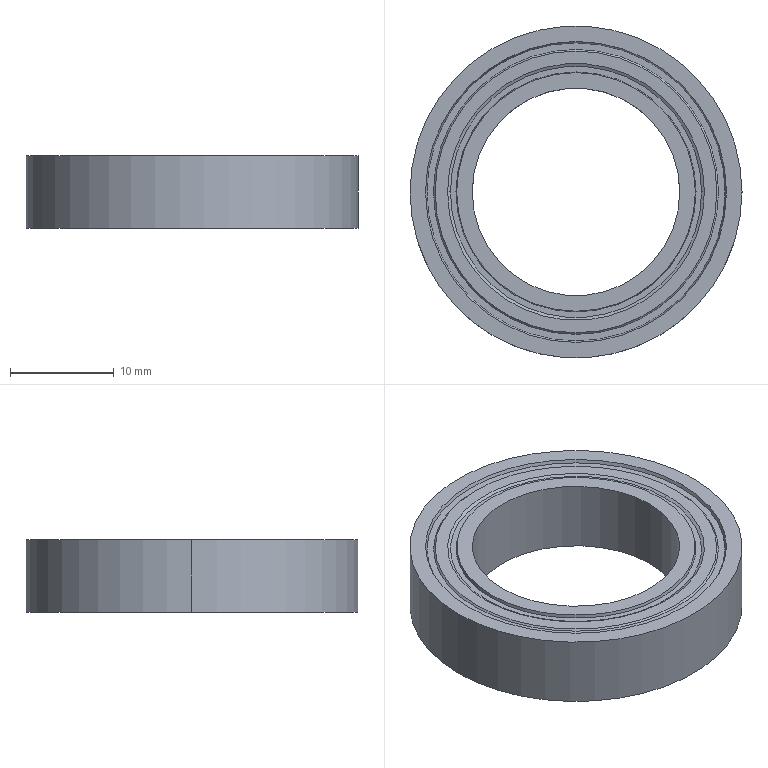Part | SolidWorks | features Extrusion 1, MirrorPattern 1, RevCut 1 | 1 solid | 30 faces | box 32 x 32 x 7 mm | volume 3321 mm3 | cone 16 | plane 10 | cylinder 4 | commonest cylinder face diameters 20 x2 32 x2
STEP:
#1=CARTESIAN_POINT('',(11.5,0.,0.));
#2=VERTEX_POINT('',#1);
#3=CARTESIAN_POINT('',(-11.5,0.,0.));
#4=VERTEX_POINT('',#3);
#5=CARTESIAN_POINT('',(0.,0.,0.));
#6=DIRECTION('',(0.,0.,-1.));
#7=DIRECTION('',(-1.,0.,0.));
#8=AXIS2_PLACEMENT_3D('',#5,#6,#7);
#9=CIRCLE('',#8,11.5);
#10=EDGE_CURVE('',#2,#4,#9,.T.);
#11=ORIENTED_EDGE('',*,*,#10,.F.);
#12=CARTESIAN_POINT('',(11.567,0.,0.3054));
#13=VERTEX_POINT('',#12);
#14=CARTESIAN_POINT('',(11.567,0.,0.3054));
#15=DIRECTION('',(0.215,0.,0.9766));
#16=VECTOR('',#15,1000.);
#17=LINE('',#14,#16);
#18=EDGE_CURVE('',#2,#13,#17,.T.);
#19=ORIENTED_EDGE('',*,*,#18,.T.);
#20=CARTESIAN_POINT('',(-11.567,0.,0.3054));
#21=VERTEX_POINT('',#20);
#22=CARTESIAN_POINT('',(0.,0.,0.3054));
#23=DIRECTION('',(0.,0.,-1.));
#24=DIRECTION('',(-1.,0.,0.));
#25=AXIS2_PLACEMENT_3D('',#22,#23,#24);
#26=CIRCLE('',#25,11.567);
#27=EDGE_CURVE('',#13,#21,#26,.T.);
#28=ORIENTED_EDGE('',*,*,#27,.T.);
#29=CARTESIAN_POINT('',(-11.567,0.,0.3054));
#30=DIRECTION('',(-0.215,0.,0.9766));
#31=VECTOR('',#30,1000.);
#32=LINE('',#29,#31);
#33=EDGE_CURVE('',#4,#21,#32,.T.);
#34=ORIENTED_EDGE('',*,*,#33,.F.);
#35=EDGE_LOOP('',(#11,#19,#28,#34));
#36=FACE_OUTER_BOUND('',#35,.T.);
#37=CARTESIAN_POINT('',(0.,0.,0.3054));
#38=DIRECTION('',(0.,0.,1.));
#39=DIRECTION('',(-1.,0.,0.));
#40=AXIS2_PLACEMENT_3D('',#37,#38,#39);
#41=CONICAL_SURFACE('',#40,11.567,0.2167);
#42=ADVANCED_FACE('',(#36),#41,.T.);
#43=CARTESIAN_POINT('',(-12.105,0.,0.3054));
#44=VERTEX_POINT('',#43);
#45=CARTESIAN_POINT('',(12.105,0.,0.3054));
#46=VERTEX_POINT('',#45);
#47=CARTESIAN_POINT('',(0.,0.,0.3054));
#48=DIRECTION('',(0.,0.,-1.));
#49=DIRECTION('',(-1.,0.,0.));
#50=AXIS2_PLACEMENT_3D('',#47,#48,#49);
#51=CIRCLE('',#50,12.105);
#52=EDGE_CURVE('',#44,#46,#51,.T.);
#53=ORIENTED_EDGE('',*,*,#52,.F.);
#54=CARTESIAN_POINT('',(-12.375,0.,0.1527));
#55=VERTEX_POINT('',#54);
#56=CARTESIAN_POINT('',(-12.375,0.,0.1527));
#57=DIRECTION('',(-0.8699,0.,-0.4932));
#58=VECTOR('',#57,1000.);
#59=LINE('',#56,#58);
#60=EDGE_CURVE('',#44,#55,#59,.T.);
#61=ORIENTED_EDGE('',*,*,#60,.T.);
#62=CARTESIAN_POINT('',(12.375,0.,0.1527));
#63=VERTEX_POINT('',#62);
#64=CARTESIAN_POINT('',(0.,0.,0.1527));
#65=DIRECTION('',(0.,0.,-1.));
#66=DIRECTION('',(-1.,0.,0.));
#67=AXIS2_PLACEMENT_3D('',#64,#65,#66);
#68=CIRCLE('',#67,12.375);
#69=EDGE_CURVE('',#55,#63,#68,.T.);
#70=ORIENTED_EDGE('',*,*,#69,.T.);
#71=CARTESIAN_POINT('',(12.375,0.,0.1527));
#72=DIRECTION('',(0.8699,0.,-0.4932));
#73=VECTOR('',#72,1000.);
#74=LINE('',#71,#73);
#75=EDGE_CURVE('',#46,#63,#74,.T.);
#76=ORIENTED_EDGE('',*,*,#75,.F.);
#77=EDGE_LOOP('',(#53,#61,#70,#76));
#78=FACE_OUTER_BOUND('',#77,.T.);
#79=CARTESIAN_POINT('',(0.,0.,0.1527));
#80=DIRECTION('',(0.,0.,-1.));
#81=DIRECTION('',(1.,0.,0.));
#82=AXIS2_PLACEMENT_3D('',#79,#80,#81);
#83=CONICAL_SURFACE('',#82,12.375,1.055);
#84=ADVANCED_FACE('',(#78),#83,.F.);
#85=CARTESIAN_POINT('',(13.575,0.,0.1527));
#86=VERTEX_POINT('',#85);
#87=CARTESIAN_POINT('',(-13.575,0.,0.1527));
#88=VERTEX_POINT('',#87);
#89=CARTESIAN_POINT('',(0.,0.,0.1527));
#90=DIRECTION('',(0.,0.,-1.));
#91=DIRECTION('',(-1.,0.,0.));
#92=AXIS2_PLACEMENT_3D('',#89,#90,#91);
#93=CIRCLE('',#92,13.575);
#94=EDGE_CURVE('',#86,#88,#93,.T.);
#95=ORIENTED_EDGE('',*,*,#94,.F.);
#96=CARTESIAN_POINT('',(13.727,0.,0.3054));
#97=VERTEX_POINT('',#96);
#98=CARTESIAN_POINT('',(13.727,0.,0.3054));
#99=DIRECTION('',(0.7071,0.,0.7071));
#100=VECTOR('',#99,1000.);
#101=LINE('',#98,#100);
#102=EDGE_CURVE('',#86,#97,#101,.T.);
#103=ORIENTED_EDGE('',*,*,#102,.T.);
#104=CARTESIAN_POINT('',(-13.727,0.,0.3054));
#105=VERTEX_POINT('',#104);
#106=CARTESIAN_POINT('',(0.,0.,0.3054));
#107=DIRECTION('',(0.,0.,-1.));
#108=DIRECTION('',(-1.,0.,0.));
#109=AXIS2_PLACEMENT_3D('',#106,#107,#108);
#110=CIRCLE('',#109,13.727);
#111=EDGE_CURVE('',#97,#105,#110,.T.);
#112=ORIENTED_EDGE('',*,*,#111,.T.);
#113=CARTESIAN_POINT('',(-13.727,0.,0.3054));
#114=DIRECTION('',(-0.7071,0.,0.7071));
#115=VECTOR('',#114,1000.);
#116=LINE('',#113,#115);
#117=EDGE_CURVE('',#88,#105,#116,.T.);
#118=ORIENTED_EDGE('',*,*,#117,.F.);
#119=EDGE_LOOP('',(#95,#103,#112,#118));
#120=FACE_OUTER_BOUND('',#119,.T.);
#121=CARTESIAN_POINT('',(0.,0.,0.3054));
#122=DIRECTION('',(0.,0.,1.));
#123=DIRECTION('',(-1.,0.,0.));
#124=AXIS2_PLACEMENT_3D('',#121,#122,#123);
#125=CONICAL_SURFACE('',#124,13.727,0.7854);
#126=ADVANCED_FACE('',(#120),#125,.T.);
#127=CARTESIAN_POINT('',(-14.366,0.,0.3054));
#128=VERTEX_POINT('',#127);
#129=CARTESIAN_POINT('',(14.366,0.,0.3054));
#130=VERTEX_POINT('',#129);
#131=CARTESIAN_POINT('',(0.,0.,0.3054));
#132=DIRECTION('',(0.,0.,-1.));
#133=DIRECTION('',(-1.,0.,0.));
#134=AXIS2_PLACEMENT_3D('',#131,#132,#133);
#135=CIRCLE('',#134,14.366);
#136=EDGE_CURVE('',#128,#130,#135,.T.);
#137=ORIENTED_EDGE('',*,*,#136,.F.);
#138=CARTESIAN_POINT('',(-14.5,0.,0.));
#139=VERTEX_POINT('',#138);
#140=CARTESIAN_POINT('',(-14.5,0.,0.));
#141=DIRECTION('',(-0.4019,0.,-0.9157));
#142=VECTOR('',#141,1000.);
#143=LINE('',#140,#142);
#144=EDGE_CURVE('',#128,#139,#143,.T.);
#145=ORIENTED_EDGE('',*,*,#144,.T.);
#146=CARTESIAN_POINT('',(14.5,0.,0.));
#147=VERTEX_POINT('',#146);
#148=CARTESIAN_POINT('',(0.,0.,0.));
#149=DIRECTION('',(0.,0.,-1.));
#150=DIRECTION('',(-1.,0.,0.));
#151=AXIS2_PLACEMENT_3D('',#148,#149,#150);
#152=CIRCLE('',#151,14.5);
#153=EDGE_CURVE('',#139,#147,#152,.T.);
#154=ORIENTED_EDGE('',*,*,#153,.T.);
#155=CARTESIAN_POINT('',(14.5,0.,0.));
#156=DIRECTION('',(0.4019,0.,-0.9157));
#157=VECTOR('',#156,1000.);
#158=LINE('',#155,#157);
#159=EDGE_CURVE('',#130,#147,#158,.T.);
#160=ORIENTED_EDGE('',*,*,#159,.F.);
#161=EDGE_LOOP('',(#137,#145,#154,#160));
#162=FACE_OUTER_BOUND('',#161,.T.);
#163=CARTESIAN_POINT('',(0.,0.,0.));
#164=DIRECTION('',(0.,0.,-1.));
#165=DIRECTION('',(1.,0.,0.));
#166=AXIS2_PLACEMENT_3D('',#163,#164,#165);
#167=CONICAL_SURFACE('',#166,14.5,0.4136);
#168=ADVANCED_FACE('',(#162),#167,.F.);
#169=CARTESIAN_POINT('',(-11.5,0.,7.));
#170=VERTEX_POINT('',#169);
#171=CARTESIAN_POINT('',(11.5,0.,7.));
#172=VERTEX_POINT('',#171);
#173=CARTESIAN_POINT('',(0.,0.,7.));
#174=DIRECTION('',(0.,0.,-1.));
#175=DIRECTION('',(-1.,0.,0.));
#176=AXIS2_PLACEMENT_3D('',#173,#174,#175);
#177=CIRCLE('',#176,11.5);
#178=EDGE_CURVE('',#170,#172,#177,.T.);
#179=ORIENTED_EDGE('',*,*,#178,.T.);
#180=CARTESIAN_POINT('',(11.567,0.,6.695));
#181=VERTEX_POINT('',#180);
#182=CARTESIAN_POINT('',(11.567,0.,6.695));
#183=DIRECTION('',(0.215,0.,-0.9766));
#184=VECTOR('',#183,1000.);
#185=LINE('',#182,#184);
#186=EDGE_CURVE('',#172,#181,#185,.T.);
#187=ORIENTED_EDGE('',*,*,#186,.T.);
#188=CARTESIAN_POINT('',(-11.567,0.,6.695));
#189=VERTEX_POINT('',#188);
#190=CARTESIAN_POINT('',(0.,0.,6.695));
#191=DIRECTION('',(0.,0.,-1.));
#192=DIRECTION('',(-1.,0.,0.));
#193=AXIS2_PLACEMENT_3D('',#190,#191,#192);
#194=CIRCLE('',#193,11.567);
#195=EDGE_CURVE('',#189,#181,#194,.T.);
#196=ORIENTED_EDGE('',*,*,#195,.F.);
#197=CARTESIAN_POINT('',(-11.567,0.,6.695));
#198=DIRECTION('',(-0.215,0.,-0.9766));
#199=VECTOR('',#198,1000.);
#200=LINE('',#197,#199);
#201=EDGE_CURVE('',#170,#189,#200,.T.);
#202=ORIENTED_EDGE('',*,*,#201,.F.);
#203=EDGE_LOOP('',(#179,#187,#196,#202));
#204=FACE_OUTER_BOUND('',#203,.T.);
#205=CARTESIAN_POINT('',(0.,0.,6.695));
#206=DIRECTION('',(0.,0.,-1.));
#207=DIRECTION('',(-1.,0.,0.));
#208=AXIS2_PLACEMENT_3D('',#205,#206,#207);
#209=CONICAL_SURFACE('',#208,11.567,0.2167);
#210=ADVANCED_FACE('',(#204),#209,.T.);
#211=CARTESIAN_POINT('',(12.105,0.,6.695));
#212=VERTEX_POINT('',#211);
#213=CARTESIAN_POINT('',(-12.105,0.,6.695));
#214=VERTEX_POINT('',#213);
#215=CARTESIAN_POINT('',(0.,0.,6.695));
#216=DIRECTION('',(0.,0.,-1.));
#217=DIRECTION('',(-1.,0.,0.));
#218=AXIS2_PLACEMENT_3D('',#215,#216,#217);
#219=CIRCLE('',#218,12.105);
#220=EDGE_CURVE('',#212,#214,#219,.T.);
#221=ORIENTED_EDGE('',*,*,#220,.T.);
#222=CARTESIAN_POINT('',(-12.375,0.,6.847));
#223=VERTEX_POINT('',#222);
#224=CARTESIAN_POINT('',(-12.375,0.,6.847));
#225=DIRECTION('',(-0.8699,0.,0.4932));
#226=VECTOR('',#225,1000.);
#227=LINE('',#224,#226);
#228=EDGE_CURVE('',#214,#223,#227,.T.);
#229=ORIENTED_EDGE('',*,*,#228,.T.);
#230=CARTESIAN_POINT('',(12.375,0.,6.847));
#231=VERTEX_POINT('',#230);
#232=CARTESIAN_POINT('',(0.,0.,6.847));
#233=DIRECTION('',(0.,0.,-1.));
#234=DIRECTION('',(-1.,0.,0.));
#235=AXIS2_PLACEMENT_3D('',#232,#233,#234);
#236=CIRCLE('',#235,12.375);
#237=EDGE_CURVE('',#231,#223,#236,.T.);
#238=ORIENTED_EDGE('',*,*,#237,.F.);
#239=CARTESIAN_POINT('',(12.375,0.,6.847));
#240=DIRECTION('',(0.8699,0.,0.4932));
#241=VECTOR('',#240,1000.);
#242=LINE('',#239,#241);
#243=EDGE_CURVE('',#212,#231,#242,.T.);
#244=ORIENTED_EDGE('',*,*,#243,.F.);
#245=EDGE_LOOP('',(#221,#229,#238,#244));
#246=FACE_OUTER_BOUND('',#245,.T.);
#247=CARTESIAN_POINT('',(0.,0.,6.847));
#248=DIRECTION('',(0.,0.,1.));
#249=DIRECTION('',(1.,0.,0.));
#250=AXIS2_PLACEMENT_3D('',#247,#248,#249);
#251=CONICAL_SURFACE('',#250,12.375,1.055);
#252=ADVANCED_FACE('',(#246),#251,.F.);
#253=CARTESIAN_POINT('',(-13.575,0.,6.847));
#254=VERTEX_POINT('',#253);
#255=CARTESIAN_POINT('',(13.575,0.,6.847));
#256=VERTEX_POINT('',#255);
#257=CARTESIAN_POINT('',(0.,0.,6.847));
#258=DIRECTION('',(0.,0.,-1.));
#259=DIRECTION('',(-1.,0.,0.));
#260=AXIS2_PLACEMENT_3D('',#257,#258,#259);
#261=CIRCLE('',#260,13.575);
#262=EDGE_CURVE('',#254,#256,#261,.T.);
#263=ORIENTED_EDGE('',*,*,#262,.T.);
#264=CARTESIAN_POINT('',(13.727,0.,6.695));
#265=VERTEX_POINT('',#264);
#266=CARTESIAN_POINT('',(13.727,0.,6.695));
#267=DIRECTION('',(0.7071,0.,-0.7071));
#268=VECTOR('',#267,1000.);
#269=LINE('',#266,#268);
#270=EDGE_CURVE('',#256,#265,#269,.T.);
#271=ORIENTED_EDGE('',*,*,#270,.T.);
#272=CARTESIAN_POINT('',(-13.727,0.,6.695));
#273=VERTEX_POINT('',#272);
#274=CARTESIAN_POINT('',(0.,0.,6.695));
#275=DIRECTION('',(0.,0.,-1.));
#276=DIRECTION('',(-1.,0.,0.));
#277=AXIS2_PLACEMENT_3D('',#274,#275,#276);
#278=CIRCLE('',#277,13.727);
#279=EDGE_CURVE('',#273,#265,#278,.T.);
#280=ORIENTED_EDGE('',*,*,#279,.F.);
#281=CARTESIAN_POINT('',(-13.727,0.,6.695));
#282=DIRECTION('',(-0.7071,0.,-0.7071));
#283=VECTOR('',#282,1000.);
#284=LINE('',#281,#283);
#285=EDGE_CURVE('',#254,#273,#284,.T.);
#286=ORIENTED_EDGE('',*,*,#285,.F.);
#287=EDGE_LOOP('',(#263,#271,#280,#286));
#288=FACE_OUTER_BOUND('',#287,.T.);
#289=CARTESIAN_POINT('',(0.,0.,6.695));
#290=DIRECTION('',(0.,0.,-1.));
#291=DIRECTION('',(-1.,0.,0.));
#292=AXIS2_PLACEMENT_3D('',#289,#290,#291);
#293=CONICAL_SURFACE('',#292,13.727,0.7854);
#294=ADVANCED_FACE('',(#288),#293,.T.);
#295=CARTESIAN_POINT('',(14.366,0.,6.695));
#296=VERTEX_POINT('',#295);
#297=CARTESIAN_POINT('',(-14.366,0.,6.695));
#298=VERTEX_POINT('',#297);
#299=CARTESIAN_POINT('',(0.,0.,6.695));
#300=DIRECTION('',(0.,0.,-1.));
#301=DIRECTION('',(-1.,0.,0.));
#302=AXIS2_PLACEMENT_3D('',#299,#300,#301);
#303=CIRCLE('',#302,14.366);
#304=EDGE_CURVE('',#296,#298,#303,.T.);
#305=ORIENTED_EDGE('',*,*,#304,.T.);
#306=CARTESIAN_POINT('',(-14.5,0.,7.));
#307=VERTEX_POINT('',#306);
#308=CARTESIAN_POINT('',(-14.5,0.,7.));
#309=DIRECTION('',(-0.4019,0.,0.9157));
#310=VECTOR('',#309,1000.);
#311=LINE('',#308,#310);
#312=EDGE_CURVE('',#298,#307,#311,.T.);
#313=ORIENTED_EDGE('',*,*,#312,.T.);
#314=CARTESIAN_POINT('',(14.5,0.,7.));
#315=VERTEX_POINT('',#314);
#316=CARTESIAN_POINT('',(0.,0.,7.));
#317=DIRECTION('',(0.,0.,-1.));
#318=DIRECTION('',(-1.,0.,0.));
#319=AXIS2_PLACEMENT_3D('',#316,#317,#318);
#320=CIRCLE('',#319,14.5);
#321=EDGE_CURVE('',#315,#307,#320,.T.);
#322=ORIENTED_EDGE('',*,*,#321,.F.);
#323=CARTESIAN_POINT('',(14.5,0.,7.));
#324=DIRECTION('',(0.4019,0.,0.9157));
#325=VECTOR('',#324,1000.);
#326=LINE('',#323,#325);
#327=EDGE_CURVE('',#296,#315,#326,.T.);
#328=ORIENTED_EDGE('',*,*,#327,.F.);
#329=EDGE_LOOP('',(#305,#313,#322,#328));
#330=FACE_OUTER_BOUND('',#329,.T.);
#331=CARTESIAN_POINT('',(0.,0.,7.));
#332=DIRECTION('',(0.,0.,1.));
#333=DIRECTION('',(1.,0.,0.));
#334=AXIS2_PLACEMENT_3D('',#331,#332,#333);
#335=CONICAL_SURFACE('',#334,14.5,0.4136);
#336=ADVANCED_FACE('',(#330),#335,.F.);
#337=CARTESIAN_POINT('',(-10.,0.,7.));
#338=VERTEX_POINT('',#337);
#339=CARTESIAN_POINT('',(10.,0.,7.));
#340=VERTEX_POINT('',#339);
#341=CARTESIAN_POINT('',(0.,0.,7.));
#342=DIRECTION('',(0.,0.,1.));
#343=DIRECTION('',(1.,0.,0.));
#344=AXIS2_PLACEMENT_3D('',#341,#342,#343);
#345=CIRCLE('',#344,10.);
#346=EDGE_CURVE('',#338,#340,#345,.T.);
#347=ORIENTED_EDGE('',*,*,#346,.T.);
#348=CARTESIAN_POINT('',(10.,0.,0.));
#349=VERTEX_POINT('',#348);
#350=CARTESIAN_POINT('',(10.,0.,7.));
#351=DIRECTION('',(0.,0.,-1.));
#352=VECTOR('',#351,1000.);
#353=LINE('',#350,#352);
#354=EDGE_CURVE('',#340,#349,#353,.T.);
#355=ORIENTED_EDGE('',*,*,#354,.T.);
#356=CARTESIAN_POINT('',(-10.,0.,0.));
#357=VERTEX_POINT('',#356);
#358=CARTESIAN_POINT('',(0.,0.,0.));
#359=DIRECTION('',(0.,0.,1.));
#360=DIRECTION('',(1.,0.,0.));
#361=AXIS2_PLACEMENT_3D('',#358,#359,#360);
#362=CIRCLE('',#361,10.);
#363=EDGE_CURVE('',#357,#349,#362,.T.);
#364=ORIENTED_EDGE('',*,*,#363,.F.);
#365=CARTESIAN_POINT('',(-10.,0.,7.));
#366=DIRECTION('',(0.,0.,-1.));
#367=VECTOR('',#366,1000.);
#368=LINE('',#365,#367);
#369=EDGE_CURVE('',#338,#357,#368,.T.);
#370=ORIENTED_EDGE('',*,*,#369,.F.);
#371=EDGE_LOOP('',(#347,#355,#364,#370));
#372=FACE_OUTER_BOUND('',#371,.T.);
#373=CARTESIAN_POINT('',(0.,0.,7.));
#374=DIRECTION('',(0.,0.,-1.));
#375=DIRECTION('',(-1.,0.,0.));
#376=AXIS2_PLACEMENT_3D('',#373,#374,#375);
#377=CYLINDRICAL_SURFACE('',#376,10.);
#378=ADVANCED_FACE('',(#372),#377,.F.);
#379=CARTESIAN_POINT('',(16.,0.,7.));
#380=VERTEX_POINT('',#379);
#381=CARTESIAN_POINT('',(-16.,0.,7.));
#382=VERTEX_POINT('',#381);
#383=CARTESIAN_POINT('',(0.,0.,7.));
#384=DIRECTION('',(0.,0.,1.));
#385=DIRECTION('',(1.,0.,0.));
#386=AXIS2_PLACEMENT_3D('',#383,#384,#385);
#387=CIRCLE('',#386,16.);
#388=EDGE_CURVE('',#380,#382,#387,.T.);
#389=ORIENTED_EDGE('',*,*,#388,.F.);
#390=CARTESIAN_POINT('',(16.,0.,0.));
#391=VERTEX_POINT('',#390);
#392=CARTESIAN_POINT('',(16.,0.,7.));
#393=DIRECTION('',(0.,0.,-1.));
#394=VECTOR('',#393,1000.);
#395=LINE('',#392,#394);
#396=EDGE_CURVE('',#380,#391,#395,.T.);
#397=ORIENTED_EDGE('',*,*,#396,.T.);
#398=CARTESIAN_POINT('',(-16.,0.,0.));
#399=VERTEX_POINT('',#398);
#400=CARTESIAN_POINT('',(0.,0.,0.));
#401=DIRECTION('',(0.,0.,1.));
#402=DIRECTION('',(1.,0.,0.));
#403=AXIS2_PLACEMENT_3D('',#400,#401,#402);
#404=CIRCLE('',#403,16.);
#405=EDGE_CURVE('',#391,#399,#404,.T.);
#406=ORIENTED_EDGE('',*,*,#405,.T.);
#407=CARTESIAN_POINT('',(-16.,0.,7.));
#408=DIRECTION('',(0.,0.,-1.));
#409=VECTOR('',#408,1000.);
#410=LINE('',#407,#409);
#411=EDGE_CURVE('',#382,#399,#410,.T.);
#412=ORIENTED_EDGE('',*,*,#411,.F.);
#413=EDGE_LOOP('',(#389,#397,#406,#412));
#414=FACE_OUTER_BOUND('',#413,.T.);
#415=CARTESIAN_POINT('',(0.,0.,7.));
#416=DIRECTION('',(0.,0.,-1.));
#417=DIRECTION('',(-1.,0.,0.));
#418=AXIS2_PLACEMENT_3D('',#415,#416,#417);
#419=CYLINDRICAL_SURFACE('',#418,16.);
#420=ADVANCED_FACE('',(#414),#419,.T.);
#421=CARTESIAN_POINT('',(0.,0.,0.));
#422=DIRECTION('',(0.,0.,1.));
#423=DIRECTION('',(1.,0.,0.));
#424=AXIS2_PLACEMENT_3D('',#421,#422,#423);
#425=CIRCLE('',#424,16.);
#426=EDGE_CURVE('',#399,#391,#425,.T.);
#427=ORIENTED_EDGE('',*,*,#426,.F.);
#428=ORIENTED_EDGE('',*,*,#405,.F.);
#429=EDGE_LOOP('',(#427,#428));
#430=FACE_OUTER_BOUND('',#429,.T.);
#431=CARTESIAN_POINT('',(0.,0.,0.));
#432=DIRECTION('',(0.,0.,-1.));
#433=DIRECTION('',(-1.,0.,0.));
#434=AXIS2_PLACEMENT_3D('',#431,#432,#433);
#435=CIRCLE('',#434,14.5);
#436=EDGE_CURVE('',#147,#139,#435,.T.);
#437=ORIENTED_EDGE('',*,*,#436,.F.);
#438=ORIENTED_EDGE('',*,*,#153,.F.);
#439=EDGE_LOOP('',(#437,#438));
#440=FACE_BOUND('',#439,.T.);
#441=CARTESIAN_POINT('',(0.,0.,0.));
#442=DIRECTION('',(0.,0.,1.));
#443=DIRECTION('',(1.,0.,0.));
#444=AXIS2_PLACEMENT_3D('',#441,#442,#443);
#445=PLANE('',#444);
#446=ADVANCED_FACE('',(#430,#440),#445,.F.);
#447=ORIENTED_EDGE('',*,*,#363,.T.);
#448=CARTESIAN_POINT('',(0.,0.,0.));
#449=DIRECTION('',(0.,0.,1.));
#450=DIRECTION('',(1.,0.,0.));
#451=AXIS2_PLACEMENT_3D('',#448,#449,#450);
#452=CIRCLE('',#451,10.);
#453=EDGE_CURVE('',#349,#357,#452,.T.);
#454=ORIENTED_EDGE('',*,*,#453,.T.);
#455=EDGE_LOOP('',(#447,#454));
#456=FACE_BOUND('',#455,.T.);
#457=CARTESIAN_POINT('',(0.,0.,0.));
#458=DIRECTION('',(0.,0.,-1.));
#459=DIRECTION('',(-1.,0.,0.));
#460=AXIS2_PLACEMENT_3D('',#457,#458,#459);
#461=CIRCLE('',#460,11.5);
#462=EDGE_CURVE('',#4,#2,#461,.T.);
#463=ORIENTED_EDGE('',*,*,#462,.T.);
#464=ORIENTED_EDGE('',*,*,#10,.T.);
#465=EDGE_LOOP('',(#463,#464));
#466=FACE_OUTER_BOUND('',#465,.T.);
#467=CARTESIAN_POINT('',(0.,0.,0.));
#468=DIRECTION('',(0.,0.,1.));
#469=DIRECTION('',(1.,0.,0.));
#470=AXIS2_PLACEMENT_3D('',#467,#468,#469);
#471=PLANE('',#470);
#472=ADVANCED_FACE('',(#456,#466),#471,.F.);
#473=CARTESIAN_POINT('',(0.,0.,7.));
#474=DIRECTION('',(0.,0.,1.));
#475=DIRECTION('',(1.,0.,0.));
#476=AXIS2_PLACEMENT_3D('',#473,#474,#475);
#477=CIRCLE('',#476,16.);
#478=EDGE_CURVE('',#382,#380,#477,.T.);
#479=ORIENTED_EDGE('',*,*,#478,.T.);
#480=ORIENTED_EDGE('',*,*,#388,.T.);
#481=EDGE_LOOP('',(#479,#480));
#482=FACE_OUTER_BOUND('',#481,.T.);
#483=ORIENTED_EDGE('',*,*,#321,.T.);
#484=CARTESIAN_POINT('',(0.,0.,7.));
#485=DIRECTION('',(0.,0.,-1.));
#486=DIRECTION('',(-1.,0.,0.));
#487=AXIS2_PLACEMENT_3D('',#484,#485,#486);
#488=CIRCLE('',#487,14.5);
#489=EDGE_CURVE('',#307,#315,#488,.T.);
#490=ORIENTED_EDGE('',*,*,#489,.T.);
#491=EDGE_LOOP('',(#483,#490));
#492=FACE_BOUND('',#491,.T.);
#493=CARTESIAN_POINT('',(0.,0.,7.));
#494=DIRECTION('',(0.,0.,1.));
#495=DIRECTION('',(1.,0.,0.));
#496=AXIS2_PLACEMENT_3D('',#493,#494,#495);
#497=PLANE('',#496);
#498=ADVANCED_FACE('',(#482,#492),#497,.T.);
#499=ORIENTED_EDGE('',*,*,#346,.F.);
#500=CARTESIAN_POINT('',(0.,0.,7.));
#501=DIRECTION('',(0.,0.,1.));
#502=DIRECTION('',(1.,0.,0.));
#503=AXIS2_PLACEMENT_3D('',#500,#501,#502);
#504=CIRCLE('',#503,10.);
#505=EDGE_CURVE('',#340,#338,#504,.T.);
#506=ORIENTED_EDGE('',*,*,#505,.F.);
#507=EDGE_LOOP('',(#499,#506));
#508=FACE_BOUND('',#507,.T.);
#509=ORIENTED_EDGE('',*,*,#178,.F.);
#510=CARTESIAN_POINT('',(0.,0.,7.));
#511=DIRECTION('',(0.,0.,-1.));
#512=DIRECTION('',(-1.,0.,0.));
#513=AXIS2_PLACEMENT_3D('',#510,#511,#512);
#514=CIRCLE('',#513,11.5);
#515=EDGE_CURVE('',#172,#170,#514,.T.);
#516=ORIENTED_EDGE('',*,*,#515,.F.);
#517=EDGE_LOOP('',(#509,#516));
#518=FACE_OUTER_BOUND('',#517,.T.);
#519=CARTESIAN_POINT('',(0.,0.,7.));
#520=DIRECTION('',(0.,0.,1.));
#521=DIRECTION('',(1.,0.,0.));
#522=AXIS2_PLACEMENT_3D('',#519,#520,#521);
#523=PLANE('',#522);
#524=ADVANCED_FACE('',(#508,#518),#523,.T.);
#525=ORIENTED_EDGE('',*,*,#396,.F.);
#526=ORIENTED_EDGE('',*,*,#478,.F.);
#527=ORIENTED_EDGE('',*,*,#411,.T.);
#528=ORIENTED_EDGE('',*,*,#426,.T.);
#529=EDGE_LOOP('',(#525,#526,#527,#528));
#530=FACE_OUTER_BOUND('',#529,.T.);
#531=CARTESIAN_POINT('',(0.,0.,7.));
#532=DIRECTION('',(0.,0.,-1.));
#533=DIRECTION('',(-1.,0.,0.));
#534=AXIS2_PLACEMENT_3D('',#531,#532,#533);
#535=CYLINDRICAL_SURFACE('',#534,16.);
#536=ADVANCED_FACE('',(#530),#535,.T.);
#537=ORIENTED_EDGE('',*,*,#354,.F.);
#538=ORIENTED_EDGE('',*,*,#505,.T.);
#539=ORIENTED_EDGE('',*,*,#369,.T.);
#540=ORIENTED_EDGE('',*,*,#453,.F.);
#541=EDGE_LOOP('',(#537,#538,#539,#540));
#542=FACE_OUTER_BOUND('',#541,.T.);
#543=CARTESIAN_POINT('',(0.,0.,7.));
#544=DIRECTION('',(0.,0.,-1.));
#545=DIRECTION('',(-1.,0.,0.));
#546=AXIS2_PLACEMENT_3D('',#543,#544,#545);
#547=CYLINDRICAL_SURFACE('',#546,10.);
#548=ADVANCED_FACE('',(#542),#547,.F.);
#549=ORIENTED_EDGE('',*,*,#312,.F.);
#550=CARTESIAN_POINT('',(0.,0.,6.695));
#551=DIRECTION('',(0.,0.,-1.));
#552=DIRECTION('',(-1.,0.,0.));
#553=AXIS2_PLACEMENT_3D('',#550,#551,#552);
#554=CIRCLE('',#553,14.366);
#555=EDGE_CURVE('',#298,#296,#554,.T.);
#556=ORIENTED_EDGE('',*,*,#555,.T.);
#557=ORIENTED_EDGE('',*,*,#327,.T.);
#558=ORIENTED_EDGE('',*,*,#489,.F.);
#559=EDGE_LOOP('',(#549,#556,#557,#558));
#560=FACE_OUTER_BOUND('',#559,.T.);
#561=CARTESIAN_POINT('',(0.,0.,7.));
#562=DIRECTION('',(0.,0.,1.));
#563=DIRECTION('',(1.,0.,0.));
#564=AXIS2_PLACEMENT_3D('',#561,#562,#563);
#565=CONICAL_SURFACE('',#564,14.5,0.4136);
#566=ADVANCED_FACE('',(#560),#565,.F.);
#567=ORIENTED_EDGE('',*,*,#279,.T.);
#568=CARTESIAN_POINT('',(0.,0.,6.695));
#569=DIRECTION('',(0.,0.,-1.));
#570=DIRECTION('',(-1.,0.,0.));
#571=AXIS2_PLACEMENT_3D('',#568,#569,#570);
#572=CIRCLE('',#571,13.727);
#573=EDGE_CURVE('',#265,#273,#572,.T.);
#574=ORIENTED_EDGE('',*,*,#573,.T.);
#575=EDGE_LOOP('',(#567,#574));
#576=FACE_BOUND('',#575,.T.);
#577=ORIENTED_EDGE('',*,*,#304,.F.);
#578=ORIENTED_EDGE('',*,*,#555,.F.);
#579=EDGE_LOOP('',(#577,#578));
#580=FACE_OUTER_BOUND('',#579,.T.);
#581=CARTESIAN_POINT('',(13.727,0.,6.695));
#582=DIRECTION('',(0.,0.,1.));
#583=DIRECTION('',(1.,0.,0.));
#584=AXIS2_PLACEMENT_3D('',#581,#582,#583);
#585=PLANE('',#584);
#586=ADVANCED_FACE('',(#576,#580),#585,.T.);
#587=ORIENTED_EDGE('',*,*,#270,.F.);
#588=CARTESIAN_POINT('',(0.,0.,6.847));
#589=DIRECTION('',(0.,0.,-1.));
#590=DIRECTION('',(-1.,0.,0.));
#591=AXIS2_PLACEMENT_3D('',#588,#589,#590);
#592=CIRCLE('',#591,13.575);
#593=EDGE_CURVE('',#256,#254,#592,.T.);
#594=ORIENTED_EDGE('',*,*,#593,.T.);
#595=ORIENTED_EDGE('',*,*,#285,.T.);
#596=ORIENTED_EDGE('',*,*,#573,.F.);
#597=EDGE_LOOP('',(#587,#594,#595,#596));
#598=FACE_OUTER_BOUND('',#597,.T.);
#599=CARTESIAN_POINT('',(0.,0.,6.695));
#600=DIRECTION('',(0.,0.,-1.));
#601=DIRECTION('',(-1.,0.,0.));
#602=AXIS2_PLACEMENT_3D('',#599,#600,#601);
#603=CONICAL_SURFACE('',#602,13.727,0.7854);
#604=ADVANCED_FACE('',(#598),#603,.T.);
#605=ORIENTED_EDGE('',*,*,#237,.T.);
#606=CARTESIAN_POINT('',(0.,0.,6.847));
#607=DIRECTION('',(0.,0.,-1.));
#608=DIRECTION('',(-1.,0.,0.));
#609=AXIS2_PLACEMENT_3D('',#606,#607,#608);
#610=CIRCLE('',#609,12.375);
#611=EDGE_CURVE('',#223,#231,#610,.T.);
#612=ORIENTED_EDGE('',*,*,#611,.T.);
#613=EDGE_LOOP('',(#605,#612));
#614=FACE_BOUND('',#613,.T.);
#615=ORIENTED_EDGE('',*,*,#262,.F.);
#616=ORIENTED_EDGE('',*,*,#593,.F.);
#617=EDGE_LOOP('',(#615,#616));
#618=FACE_OUTER_BOUND('',#617,.T.);
#619=CARTESIAN_POINT('',(12.375,0.,6.847));
#620=DIRECTION('',(0.,0.,1.));
#621=DIRECTION('',(1.,0.,0.));
#622=AXIS2_PLACEMENT_3D('',#619,#620,#621);
#623=PLANE('',#622);
#624=ADVANCED_FACE('',(#614,#618),#623,.T.);
#625=ORIENTED_EDGE('',*,*,#228,.F.);
#626=CARTESIAN_POINT('',(0.,0.,6.695));
#627=DIRECTION('',(0.,0.,-1.));
#628=DIRECTION('',(-1.,0.,0.));
#629=AXIS2_PLACEMENT_3D('',#626,#627,#628);
#630=CIRCLE('',#629,12.105);
#631=EDGE_CURVE('',#214,#212,#630,.T.);
#632=ORIENTED_EDGE('',*,*,#631,.T.);
#633=ORIENTED_EDGE('',*,*,#243,.T.);
#634=ORIENTED_EDGE('',*,*,#611,.F.);
#635=EDGE_LOOP('',(#625,#632,#633,#634));
#636=FACE_OUTER_BOUND('',#635,.T.);
#637=CARTESIAN_POINT('',(0.,0.,6.847));
#638=DIRECTION('',(0.,0.,1.));
#639=DIRECTION('',(1.,0.,0.));
#640=AXIS2_PLACEMENT_3D('',#637,#638,#639);
#641=CONICAL_SURFACE('',#640,12.375,1.055);
#642=ADVANCED_FACE('',(#636),#641,.F.);
#643=ORIENTED_EDGE('',*,*,#195,.T.);
#644=CARTESIAN_POINT('',(0.,0.,6.695));
#645=DIRECTION('',(0.,0.,-1.));
#646=DIRECTION('',(-1.,0.,0.));
#647=AXIS2_PLACEMENT_3D('',#644,#645,#646);
#648=CIRCLE('',#647,11.567);
#649=EDGE_CURVE('',#181,#189,#648,.T.);
#650=ORIENTED_EDGE('',*,*,#649,.T.);
#651=EDGE_LOOP('',(#643,#650));
#652=FACE_BOUND('',#651,.T.);
#653=ORIENTED_EDGE('',*,*,#220,.F.);
#654=ORIENTED_EDGE('',*,*,#631,.F.);
#655=EDGE_LOOP('',(#653,#654));
#656=FACE_OUTER_BOUND('',#655,.T.);
#657=CARTESIAN_POINT('',(11.567,0.,6.695));
#658=DIRECTION('',(0.,0.,1.));
#659=DIRECTION('',(1.,0.,0.));
#660=AXIS2_PLACEMENT_3D('',#657,#658,#659);
#661=PLANE('',#660);
#662=ADVANCED_FACE('',(#652,#656),#661,.T.);
#663=ORIENTED_EDGE('',*,*,#186,.F.);
#664=ORIENTED_EDGE('',*,*,#515,.T.);
#665=ORIENTED_EDGE('',*,*,#201,.T.);
#666=ORIENTED_EDGE('',*,*,#649,.F.);
#667=EDGE_LOOP('',(#663,#664,#665,#666));
#668=FACE_OUTER_BOUND('',#667,.T.);
#669=CARTESIAN_POINT('',(0.,0.,6.695));
#670=DIRECTION('',(0.,0.,-1.));
#671=DIRECTION('',(-1.,0.,0.));
#672=AXIS2_PLACEMENT_3D('',#669,#670,#671);
#673=CONICAL_SURFACE('',#672,11.567,0.2167);
#674=ADVANCED_FACE('',(#668),#673,.T.);
#675=ORIENTED_EDGE('',*,*,#144,.F.);
#676=CARTESIAN_POINT('',(0.,0.,0.3054));
#677=DIRECTION('',(0.,0.,-1.));
#678=DIRECTION('',(-1.,0.,0.));
#679=AXIS2_PLACEMENT_3D('',#676,#677,#678);
#680=CIRCLE('',#679,14.366);
#681=EDGE_CURVE('',#130,#128,#680,.T.);
#682=ORIENTED_EDGE('',*,*,#681,.F.);
#683=ORIENTED_EDGE('',*,*,#159,.T.);
#684=ORIENTED_EDGE('',*,*,#436,.T.);
#685=EDGE_LOOP('',(#675,#682,#683,#684));
#686=FACE_OUTER_BOUND('',#685,.T.);
#687=CARTESIAN_POINT('',(0.,0.,0.));
#688=DIRECTION('',(0.,0.,-1.));
#689=DIRECTION('',(1.,0.,0.));
#690=AXIS2_PLACEMENT_3D('',#687,#688,#689);
#691=CONICAL_SURFACE('',#690,14.5,0.4136);
#692=ADVANCED_FACE('',(#686),#691,.F.);
#693=CARTESIAN_POINT('',(0.,0.,0.3054));
#694=DIRECTION('',(0.,0.,-1.));
#695=DIRECTION('',(-1.,0.,0.));
#696=AXIS2_PLACEMENT_3D('',#693,#694,#695);
#697=CIRCLE('',#696,13.727);
#698=EDGE_CURVE('',#105,#97,#697,.T.);
#699=ORIENTED_EDGE('',*,*,#698,.F.);
#700=ORIENTED_EDGE('',*,*,#111,.F.);
#701=EDGE_LOOP('',(#699,#700));
#702=FACE_BOUND('',#701,.T.);
#703=ORIENTED_EDGE('',*,*,#681,.T.);
#704=ORIENTED_EDGE('',*,*,#136,.T.);
#705=EDGE_LOOP('',(#703,#704));
#706=FACE_OUTER_BOUND('',#705,.T.);
#707=CARTESIAN_POINT('',(13.727,0.,0.3054));
#708=DIRECTION('',(0.,0.,-1.));
#709=DIRECTION('',(1.,0.,0.));
#710=AXIS2_PLACEMENT_3D('',#707,#708,#709);
#711=PLANE('',#710);
#712=ADVANCED_FACE('',(#702,#706),#711,.T.);
#713=ORIENTED_EDGE('',*,*,#102,.F.);
#714=CARTESIAN_POINT('',(0.,0.,0.1527));
#715=DIRECTION('',(0.,0.,-1.));
#716=DIRECTION('',(-1.,0.,0.));
#717=AXIS2_PLACEMENT_3D('',#714,#715,#716);
#718=CIRCLE('',#717,13.575);
#719=EDGE_CURVE('',#88,#86,#718,.T.);
#720=ORIENTED_EDGE('',*,*,#719,.F.);
#721=ORIENTED_EDGE('',*,*,#117,.T.);
#722=ORIENTED_EDGE('',*,*,#698,.T.);
#723=EDGE_LOOP('',(#713,#720,#721,#722));
#724=FACE_OUTER_BOUND('',#723,.T.);
#725=CARTESIAN_POINT('',(0.,0.,0.3054));
#726=DIRECTION('',(0.,0.,1.));
#727=DIRECTION('',(-1.,0.,0.));
#728=AXIS2_PLACEMENT_3D('',#725,#726,#727);
#729=CONICAL_SURFACE('',#728,13.727,0.7854);
#730=ADVANCED_FACE('',(#724),#729,.T.);
#731=CARTESIAN_POINT('',(0.,0.,0.1527));
#732=DIRECTION('',(0.,0.,-1.));
#733=DIRECTION('',(-1.,0.,0.));
#734=AXIS2_PLACEMENT_3D('',#731,#732,#733);
#735=CIRCLE('',#734,12.375);
#736=EDGE_CURVE('',#63,#55,#735,.T.);
#737=ORIENTED_EDGE('',*,*,#736,.F.);
#738=ORIENTED_EDGE('',*,*,#69,.F.);
#739=EDGE_LOOP('',(#737,#738));
#740=FACE_BOUND('',#739,.T.);
#741=ORIENTED_EDGE('',*,*,#719,.T.);
#742=ORIENTED_EDGE('',*,*,#94,.T.);
#743=EDGE_LOOP('',(#741,#742));
#744=FACE_OUTER_BOUND('',#743,.T.);
#745=CARTESIAN_POINT('',(12.375,0.,0.1527));
#746=DIRECTION('',(0.,0.,-1.));
#747=DIRECTION('',(1.,0.,0.));
#748=AXIS2_PLACEMENT_3D('',#745,#746,#747);
#749=PLANE('',#748);
#750=ADVANCED_FACE('',(#740,#744),#749,.T.);
#751=ORIENTED_EDGE('',*,*,#60,.F.);
#752=CARTESIAN_POINT('',(0.,0.,0.3054));
#753=DIRECTION('',(0.,0.,-1.));
#754=DIRECTION('',(-1.,0.,0.));
#755=AXIS2_PLACEMENT_3D('',#752,#753,#754);
#756=CIRCLE('',#755,12.105);
#757=EDGE_CURVE('',#46,#44,#756,.T.);
#758=ORIENTED_EDGE('',*,*,#757,.F.);
#759=ORIENTED_EDGE('',*,*,#75,.T.);
#760=ORIENTED_EDGE('',*,*,#736,.T.);
#761=EDGE_LOOP('',(#751,#758,#759,#760));
#762=FACE_OUTER_BOUND('',#761,.T.);
#763=CARTESIAN_POINT('',(0.,0.,0.1527));
#764=DIRECTION('',(0.,0.,-1.));
#765=DIRECTION('',(1.,0.,0.));
#766=AXIS2_PLACEMENT_3D('',#763,#764,#765);
#767=CONICAL_SURFACE('',#766,12.375,1.055);
#768=ADVANCED_FACE('',(#762),#767,.F.);
#769=CARTESIAN_POINT('',(0.,0.,0.3054));
#770=DIRECTION('',(0.,0.,-1.));
#771=DIRECTION('',(-1.,0.,0.));
#772=AXIS2_PLACEMENT_3D('',#769,#770,#771);
#773=CIRCLE('',#772,11.567);
#774=EDGE_CURVE('',#21,#13,#773,.T.);
#775=ORIENTED_EDGE('',*,*,#774,.F.);
#776=ORIENTED_EDGE('',*,*,#27,.F.);
#777=EDGE_LOOP('',(#775,#776));
#778=FACE_BOUND('',#777,.T.);
#779=ORIENTED_EDGE('',*,*,#757,.T.);
#780=ORIENTED_EDGE('',*,*,#52,.T.);
#781=EDGE_LOOP('',(#779,#780));
#782=FACE_OUTER_BOUND('',#781,.T.);
#783=CARTESIAN_POINT('',(11.567,0.,0.3054));
#784=DIRECTION('',(0.,0.,-1.));
#785=DIRECTION('',(1.,0.,0.));
#786=AXIS2_PLACEMENT_3D('',#783,#784,#785);
#787=PLANE('',#786);
#788=ADVANCED_FACE('',(#778,#782),#787,.T.);
#789=ORIENTED_EDGE('',*,*,#18,.F.);
#790=ORIENTED_EDGE('',*,*,#462,.F.);
#791=ORIENTED_EDGE('',*,*,#33,.T.);
#792=ORIENTED_EDGE('',*,*,#774,.T.);
#793=EDGE_LOOP('',(#789,#790,#791,#792));
#794=FACE_OUTER_BOUND('',#793,.T.);
#795=CARTESIAN_POINT('',(0.,0.,0.3054));
#796=DIRECTION('',(0.,0.,1.));
#797=DIRECTION('',(-1.,0.,0.));
#798=AXIS2_PLACEMENT_3D('',#795,#796,#797);
#799=CONICAL_SURFACE('',#798,11.567,0.2167);
#800=ADVANCED_FACE('',(#794),#799,.T.);
#801=CLOSED_SHELL('',(#42,#84,#126,#168,#210,#252,#294,#336,#378,#420,#446,#472,#498,#524,#536,#548,#566,#586,#604,#624,#642,#662,#674,#692,#712,#730,#750,#768,#788,#800));
#802=MANIFOLD_SOLID_BREP('',#801);
#803=CARTESIAN_POINT('',(0.,0.,0.));
#804=DIRECTION('',(0.,0.,1.));
#805=DIRECTION('',(1.,0.,0.));
#806=AXIS2_PLACEMENT_3D('',#803,#804,#805);
#807=(LENGTH_UNIT()NAMED_UNIT(*)SI_UNIT(.MILLI.,.METRE.));
#808=UNCERTAINTY_MEASURE_WITH_UNIT(LENGTH_MEASURE(0.00001),#807,'','');
#809=(NAMED_UNIT(*)PLANE_ANGLE_UNIT()SI_UNIT($,.RADIAN.));
#810=(NAMED_UNIT(*)SI_UNIT($,.STERADIAN.)SOLID_ANGLE_UNIT());
#811=(GEOMETRIC_REPRESENTATION_CONTEXT(3)GLOBAL_UNCERTAINTY_ASSIGNED_CONTEXT((#808))GLOBAL_UNIT_ASSIGNED_CONTEXT((#807,#809,#810))REPRESENTATION_CONTEXT('',''));
#812=ADVANCED_BREP_SHAPE_REPRESENTATION('',(#802,#806),#811);